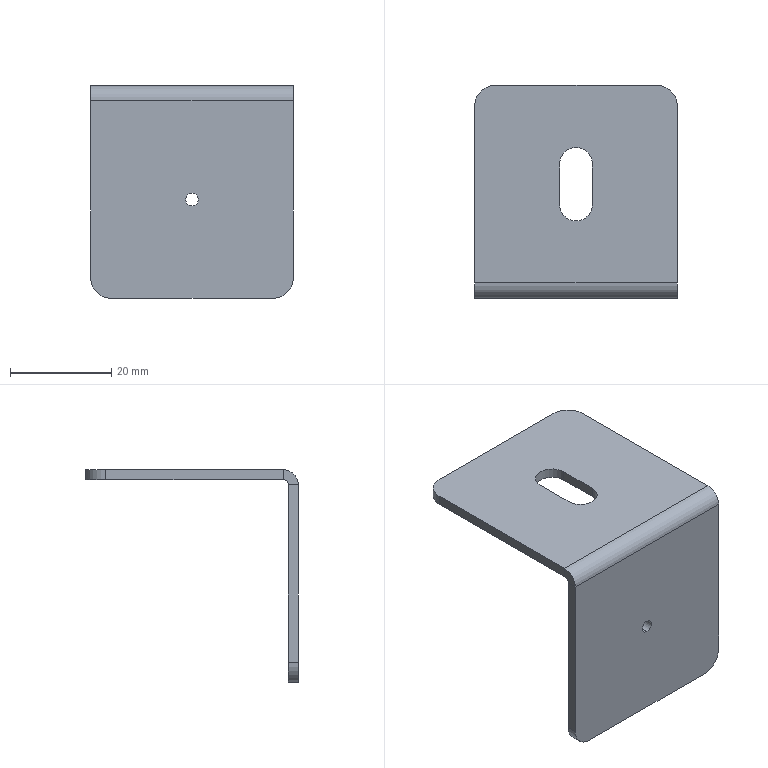Part | SolidWorks | features EdgeFlange 1, Fillet 1, FlatPattern 1, HoleWzd 1, ICE 1, SMBaseFlange 1, SheetMetal 1 | 1 solid | 24 faces | box 40 x 42 x 42 mm | volume 6284 mm3 | plane 14 | cylinder 10 | commonest cylinder face diameters 8 x4 2.5 x2 6.5 x2 2 x1 6 x1
STEP:
#1=CARTESIAN_POINT('',(0.,0.,-2.75));
#2=VERTEX_POINT('',#1);
#3=CARTESIAN_POINT('',(0.,0.,-0.25));
#4=VERTEX_POINT('',#3);
#5=CARTESIAN_POINT('',(0.,0.,-1.5));
#6=DIRECTION('',(0.,1.,0.));
#7=DIRECTION('',(0.,0.,1.));
#8=AXIS2_PLACEMENT_3D('',#5,#6,#7);
#9=CIRCLE('',#8,1.25);
#10=EDGE_CURVE('',#2,#4,#9,.T.);
#11=ORIENTED_EDGE('',*,*,#10,.T.);
#12=CARTESIAN_POINT('',(0.,-2.,-0.25));
#13=VERTEX_POINT('',#12);
#14=CARTESIAN_POINT('',(0.,-2.,-0.25));
#15=DIRECTION('',(0.,-1.,0.));
#16=VECTOR('',#15,1000.);
#17=LINE('',#14,#16);
#18=EDGE_CURVE('',#4,#13,#17,.T.);
#19=ORIENTED_EDGE('',*,*,#18,.T.);
#20=CARTESIAN_POINT('',(0.,-2.,-2.75));
#21=VERTEX_POINT('',#20);
#22=CARTESIAN_POINT('',(0.,-2.,-1.5));
#23=DIRECTION('',(0.,-1.,0.));
#24=DIRECTION('',(0.,0.,-1.));
#25=AXIS2_PLACEMENT_3D('',#22,#23,#24);
#26=CIRCLE('',#25,1.25);
#27=EDGE_CURVE('',#13,#21,#26,.T.);
#28=ORIENTED_EDGE('',*,*,#27,.T.);
#29=CARTESIAN_POINT('',(0.,-2.,-2.75));
#30=DIRECTION('',(0.,-1.,0.));
#31=VECTOR('',#30,1000.);
#32=LINE('',#29,#31);
#33=EDGE_CURVE('',#2,#21,#32,.T.);
#34=ORIENTED_EDGE('',*,*,#33,.F.);
#35=EDGE_LOOP('',(#11,#19,#28,#34));
#36=FACE_OUTER_BOUND('',#35,.T.);
#37=CARTESIAN_POINT('',(0.,-2.,-1.5));
#38=DIRECTION('',(0.,-1.,0.));
#39=DIRECTION('',(0.,0.,-1.));
#40=AXIS2_PLACEMENT_3D('',#37,#38,#39);
#41=CYLINDRICAL_SURFACE('',#40,1.25);
#42=ADVANCED_FACE('',(#36),#41,.F.);
#43=CARTESIAN_POINT('',(20.,-2.,18.));
#44=VERTEX_POINT('',#43);
#45=CARTESIAN_POINT('',(20.,-2.,-17.));
#46=VERTEX_POINT('',#45);
#47=CARTESIAN_POINT('',(20.,-2.,-21.));
#48=DIRECTION('',(0.,0.,-1.));
#49=VECTOR('',#48,1000.);
#50=LINE('',#47,#49);
#51=EDGE_CURVE('',#44,#46,#50,.T.);
#52=ORIENTED_EDGE('',*,*,#51,.T.);
#53=CARTESIAN_POINT('',(20.,0.,-17.));
#54=VERTEX_POINT('',#53);
#55=CARTESIAN_POINT('',(20.,-2.,-17.));
#56=DIRECTION('',(0.,1.,0.));
#57=VECTOR('',#56,1000.);
#58=LINE('',#55,#57);
#59=EDGE_CURVE('',#46,#54,#58,.T.);
#60=ORIENTED_EDGE('',*,*,#59,.T.);
#61=CARTESIAN_POINT('',(20.,0.,18.));
#62=VERTEX_POINT('',#61);
#63=CARTESIAN_POINT('',(20.,0.,-21.));
#64=DIRECTION('',(0.,0.,-1.));
#65=VECTOR('',#64,1000.);
#66=LINE('',#63,#65);
#67=EDGE_CURVE('',#62,#54,#66,.T.);
#68=ORIENTED_EDGE('',*,*,#67,.F.);
#69=CARTESIAN_POINT('',(20.,0.,18.));
#70=DIRECTION('',(0.,-1.,0.));
#71=VECTOR('',#70,1000.);
#72=LINE('',#69,#71);
#73=EDGE_CURVE('',#62,#44,#72,.T.);
#74=ORIENTED_EDGE('',*,*,#73,.T.);
#75=EDGE_LOOP('',(#52,#60,#68,#74));
#76=FACE_OUTER_BOUND('',#75,.T.);
#77=CARTESIAN_POINT('',(20.,-2.,-21.));
#78=DIRECTION('',(1.,0.,0.));
#79=DIRECTION('',(0.,0.,-1.));
#80=AXIS2_PLACEMENT_3D('',#77,#78,#79);
#81=PLANE('',#80);
#82=ADVANCED_FACE('',(#76),#81,.T.);
#83=CARTESIAN_POINT('',(0.,-2.,-1.5));
#84=DIRECTION('',(0.,-1.,0.));
#85=DIRECTION('',(0.,0.,-1.));
#86=AXIS2_PLACEMENT_3D('',#83,#84,#85);
#87=CIRCLE('',#86,1.25);
#88=EDGE_CURVE('',#21,#13,#87,.T.);
#89=ORIENTED_EDGE('',*,*,#88,.F.);
#90=ORIENTED_EDGE('',*,*,#27,.F.);
#91=EDGE_LOOP('',(#89,#90));
#92=FACE_BOUND('',#91,.T.);
#93=CARTESIAN_POINT('',(-20.,-2.,-17.));
#94=VERTEX_POINT('',#93);
#95=CARTESIAN_POINT('',(-20.,-2.,18.));
#96=VERTEX_POINT('',#95);
#97=CARTESIAN_POINT('',(-20.,-2.,-21.));
#98=DIRECTION('',(0.,0.,1.));
#99=VECTOR('',#98,1000.);
#100=LINE('',#97,#99);
#101=EDGE_CURVE('',#94,#96,#100,.T.);
#102=ORIENTED_EDGE('',*,*,#101,.F.);
#103=CARTESIAN_POINT('',(-16.,-2.,-21.));
#104=VERTEX_POINT('',#103);
#105=CARTESIAN_POINT('',(-16.,-2.,-17.));
#106=DIRECTION('',(0.,-1.,0.));
#107=DIRECTION('',(0.,0.,1.));
#108=AXIS2_PLACEMENT_3D('',#105,#106,#107);
#109=CIRCLE('',#108,4.);
#110=EDGE_CURVE('',#94,#104,#109,.T.);
#111=ORIENTED_EDGE('',*,*,#110,.T.);
#112=CARTESIAN_POINT('',(16.,-2.,-21.));
#113=VERTEX_POINT('',#112);
#114=CARTESIAN_POINT('',(-20.,-2.,-21.));
#115=DIRECTION('',(-1.,0.,0.));
#116=VECTOR('',#115,1000.);
#117=LINE('',#114,#116);
#118=EDGE_CURVE('',#113,#104,#117,.T.);
#119=ORIENTED_EDGE('',*,*,#118,.F.);
#120=CARTESIAN_POINT('',(16.,-2.,-17.));
#121=DIRECTION('',(0.,-1.,0.));
#122=DIRECTION('',(0.,0.,1.));
#123=AXIS2_PLACEMENT_3D('',#120,#121,#122);
#124=CIRCLE('',#123,4.);
#125=EDGE_CURVE('',#113,#46,#124,.T.);
#126=ORIENTED_EDGE('',*,*,#125,.T.);
#127=ORIENTED_EDGE('',*,*,#51,.F.);
#128=CARTESIAN_POINT('',(20.,-2.,18.));
#129=DIRECTION('',(-1.,0.,0.));
#130=VECTOR('',#129,1000.);
#131=LINE('',#128,#130);
#132=EDGE_CURVE('',#44,#96,#131,.T.);
#133=ORIENTED_EDGE('',*,*,#132,.T.);
#134=EDGE_LOOP('',(#102,#111,#119,#126,#127,#133));
#135=FACE_OUTER_BOUND('',#134,.T.);
#136=CARTESIAN_POINT('',(0.,-2.,0.));
#137=DIRECTION('',(0.,1.,0.));
#138=DIRECTION('',(0.,0.,1.));
#139=AXIS2_PLACEMENT_3D('',#136,#137,#138);
#140=PLANE('',#139);
#141=ADVANCED_FACE('',(#92,#135),#140,.F.);
#142=ORIENTED_EDGE('',*,*,#10,.F.);
#143=CARTESIAN_POINT('',(0.,0.,-1.5));
#144=DIRECTION('',(0.,1.,0.));
#145=DIRECTION('',(0.,0.,1.));
#146=AXIS2_PLACEMENT_3D('',#143,#144,#145);
#147=CIRCLE('',#146,1.25);
#148=EDGE_CURVE('',#4,#2,#147,.T.);
#149=ORIENTED_EDGE('',*,*,#148,.F.);
#150=EDGE_LOOP('',(#142,#149));
#151=FACE_BOUND('',#150,.T.);
#152=CARTESIAN_POINT('',(16.,0.,-21.));
#153=VERTEX_POINT('',#152);
#154=CARTESIAN_POINT('',(-16.,0.,-21.));
#155=VERTEX_POINT('',#154);
#156=CARTESIAN_POINT('',(-20.,0.,-21.));
#157=DIRECTION('',(-1.,0.,0.));
#158=VECTOR('',#157,1000.);
#159=LINE('',#156,#158);
#160=EDGE_CURVE('',#153,#155,#159,.T.);
#161=ORIENTED_EDGE('',*,*,#160,.T.);
#162=CARTESIAN_POINT('',(-20.,0.,-17.));
#163=VERTEX_POINT('',#162);
#164=CARTESIAN_POINT('',(-16.,0.,-17.));
#165=DIRECTION('',(0.,1.,0.));
#166=DIRECTION('',(0.,0.,1.));
#167=AXIS2_PLACEMENT_3D('',#164,#165,#166);
#168=CIRCLE('',#167,4.);
#169=EDGE_CURVE('',#155,#163,#168,.T.);
#170=ORIENTED_EDGE('',*,*,#169,.T.);
#171=CARTESIAN_POINT('',(-20.,0.,18.));
#172=VERTEX_POINT('',#171);
#173=CARTESIAN_POINT('',(-20.,0.,-21.));
#174=DIRECTION('',(0.,0.,1.));
#175=VECTOR('',#174,1000.);
#176=LINE('',#173,#175);
#177=EDGE_CURVE('',#163,#172,#176,.T.);
#178=ORIENTED_EDGE('',*,*,#177,.T.);
#179=CARTESIAN_POINT('',(20.,0.,18.));
#180=DIRECTION('',(-1.,0.,0.));
#181=VECTOR('',#180,1000.);
#182=LINE('',#179,#181);
#183=EDGE_CURVE('',#62,#172,#182,.T.);
#184=ORIENTED_EDGE('',*,*,#183,.F.);
#185=ORIENTED_EDGE('',*,*,#67,.T.);
#186=CARTESIAN_POINT('',(16.,0.,-17.));
#187=DIRECTION('',(0.,1.,0.));
#188=DIRECTION('',(0.,0.,1.));
#189=AXIS2_PLACEMENT_3D('',#186,#187,#188);
#190=CIRCLE('',#189,4.);
#191=EDGE_CURVE('',#54,#153,#190,.T.);
#192=ORIENTED_EDGE('',*,*,#191,.T.);
#193=EDGE_LOOP('',(#161,#170,#178,#184,#185,#192));
#194=FACE_OUTER_BOUND('',#193,.T.);
#195=CARTESIAN_POINT('',(0.,0.,0.));
#196=DIRECTION('',(0.,1.,0.));
#197=DIRECTION('',(0.,0.,1.));
#198=AXIS2_PLACEMENT_3D('',#195,#196,#197);
#199=PLANE('',#198);
#200=ADVANCED_FACE('',(#151,#194),#199,.T.);
#201=ORIENTED_EDGE('',*,*,#177,.F.);
#202=CARTESIAN_POINT('',(-20.,-2.,-17.));
#203=DIRECTION('',(0.,-1.,0.));
#204=VECTOR('',#203,1000.);
#205=LINE('',#202,#204);
#206=EDGE_CURVE('',#163,#94,#205,.T.);
#207=ORIENTED_EDGE('',*,*,#206,.T.);
#208=ORIENTED_EDGE('',*,*,#101,.T.);
#209=CARTESIAN_POINT('',(-20.,0.,18.));
#210=DIRECTION('',(0.,-1.,0.));
#211=VECTOR('',#210,1000.);
#212=LINE('',#209,#211);
#213=EDGE_CURVE('',#172,#96,#212,.T.);
#214=ORIENTED_EDGE('',*,*,#213,.F.);
#215=EDGE_LOOP('',(#201,#207,#208,#214));
#216=FACE_OUTER_BOUND('',#215,.T.);
#217=CARTESIAN_POINT('',(-20.,-2.,-21.));
#218=DIRECTION('',(-1.,0.,0.));
#219=DIRECTION('',(0.,0.,1.));
#220=AXIS2_PLACEMENT_3D('',#217,#218,#219);
#221=PLANE('',#220);
#222=ADVANCED_FACE('',(#216),#221,.T.);
#223=ORIENTED_EDGE('',*,*,#118,.T.);
#224=CARTESIAN_POINT('',(-16.,-2.,-21.));
#225=DIRECTION('',(0.,1.,0.));
#226=VECTOR('',#225,1000.);
#227=LINE('',#224,#226);
#228=EDGE_CURVE('',#104,#155,#227,.T.);
#229=ORIENTED_EDGE('',*,*,#228,.T.);
#230=ORIENTED_EDGE('',*,*,#160,.F.);
#231=CARTESIAN_POINT('',(16.,-2.,-21.));
#232=DIRECTION('',(0.,-1.,0.));
#233=VECTOR('',#232,1000.);
#234=LINE('',#231,#233);
#235=EDGE_CURVE('',#153,#113,#234,.T.);
#236=ORIENTED_EDGE('',*,*,#235,.T.);
#237=EDGE_LOOP('',(#223,#229,#230,#236));
#238=FACE_OUTER_BOUND('',#237,.T.);
#239=CARTESIAN_POINT('',(-20.,-2.,-21.));
#240=DIRECTION('',(0.,0.,-1.));
#241=DIRECTION('',(-1.,0.,0.));
#242=AXIS2_PLACEMENT_3D('',#239,#240,#241);
#243=PLANE('',#242);
#244=ADVANCED_FACE('',(#238),#243,.T.);
#245=CARTESIAN_POINT('',(-20.,1.,19.));
#246=VERTEX_POINT('',#245);
#247=CARTESIAN_POINT('',(-20.,1.,21.));
#248=VERTEX_POINT('',#247);
#249=CARTESIAN_POINT('',(-20.,1.,21.));
#250=DIRECTION('',(0.,0.,1.));
#251=VECTOR('',#250,1000.);
#252=LINE('',#249,#251);
#253=EDGE_CURVE('',#246,#248,#252,.T.);
#254=ORIENTED_EDGE('',*,*,#253,.F.);
#255=CARTESIAN_POINT('',(-20.,1.,18.));
#256=DIRECTION('',(-1.,0.,0.));
#257=DIRECTION('',(0.,0.,-1.));
#258=AXIS2_PLACEMENT_3D('',#255,#256,#257);
#259=CIRCLE('',#258,1.);
#260=EDGE_CURVE('',#172,#246,#259,.T.);
#261=ORIENTED_EDGE('',*,*,#260,.F.);
#262=ORIENTED_EDGE('',*,*,#213,.T.);
#263=CARTESIAN_POINT('',(-20.,1.,18.));
#264=DIRECTION('',(-1.,0.,0.));
#265=DIRECTION('',(0.,0.,-1.));
#266=AXIS2_PLACEMENT_3D('',#263,#264,#265);
#267=CIRCLE('',#266,3.);
#268=EDGE_CURVE('',#96,#248,#267,.T.);
#269=ORIENTED_EDGE('',*,*,#268,.T.);
#270=EDGE_LOOP('',(#254,#261,#262,#269));
#271=FACE_OUTER_BOUND('',#270,.T.);
#272=CARTESIAN_POINT('',(-20.,1.,18.));
#273=DIRECTION('',(-1.,0.,0.));
#274=DIRECTION('',(0.,0.,1.));
#275=AXIS2_PLACEMENT_3D('',#272,#273,#274);
#276=PLANE('',#275);
#277=ADVANCED_FACE('',(#271),#276,.T.);
#278=CARTESIAN_POINT('',(20.,1.,19.));
#279=VERTEX_POINT('',#278);
#280=CARTESIAN_POINT('',(20.,1.,18.));
#281=DIRECTION('',(1.,0.,0.));
#282=DIRECTION('',(0.,0.,-1.));
#283=AXIS2_PLACEMENT_3D('',#280,#281,#282);
#284=CIRCLE('',#283,1.);
#285=EDGE_CURVE('',#279,#62,#284,.T.);
#286=ORIENTED_EDGE('',*,*,#285,.F.);
#287=CARTESIAN_POINT('',(20.,1.,21.));
#288=VERTEX_POINT('',#287);
#289=CARTESIAN_POINT('',(20.,1.,19.));
#290=DIRECTION('',(0.,0.,1.));
#291=VECTOR('',#290,1000.);
#292=LINE('',#289,#291);
#293=EDGE_CURVE('',#279,#288,#292,.T.);
#294=ORIENTED_EDGE('',*,*,#293,.T.);
#295=CARTESIAN_POINT('',(20.,1.,18.));
#296=DIRECTION('',(1.,0.,0.));
#297=DIRECTION('',(0.,0.,-1.));
#298=AXIS2_PLACEMENT_3D('',#295,#296,#297);
#299=CIRCLE('',#298,3.);
#300=EDGE_CURVE('',#288,#44,#299,.T.);
#301=ORIENTED_EDGE('',*,*,#300,.T.);
#302=ORIENTED_EDGE('',*,*,#73,.F.);
#303=EDGE_LOOP('',(#286,#294,#301,#302));
#304=FACE_OUTER_BOUND('',#303,.T.);
#305=CARTESIAN_POINT('',(20.,1.,18.));
#306=DIRECTION('',(-1.,0.,0.));
#307=DIRECTION('',(0.,0.,1.));
#308=AXIS2_PLACEMENT_3D('',#305,#306,#307);
#309=PLANE('',#308);
#310=ADVANCED_FACE('',(#304),#309,.F.);
#311=ORIENTED_EDGE('',*,*,#132,.F.);
#312=ORIENTED_EDGE('',*,*,#300,.F.);
#313=CARTESIAN_POINT('',(-20.,1.,21.));
#314=DIRECTION('',(-1.,0.,0.));
#315=VECTOR('',#314,1000.);
#316=LINE('',#313,#315);
#317=EDGE_CURVE('',#288,#248,#316,.T.);
#318=ORIENTED_EDGE('',*,*,#317,.T.);
#319=ORIENTED_EDGE('',*,*,#268,.F.);
#320=EDGE_LOOP('',(#311,#312,#318,#319));
#321=FACE_OUTER_BOUND('',#320,.T.);
#322=CARTESIAN_POINT('',(20.,1.,18.));
#323=DIRECTION('',(1.,0.,0.));
#324=DIRECTION('',(0.,0.,1.));
#325=AXIS2_PLACEMENT_3D('',#322,#323,#324);
#326=CYLINDRICAL_SURFACE('',#325,3.);
#327=ADVANCED_FACE('',(#321),#326,.T.);
#328=ORIENTED_EDGE('',*,*,#183,.T.);
#329=ORIENTED_EDGE('',*,*,#260,.T.);
#330=CARTESIAN_POINT('',(-20.,1.,19.));
#331=DIRECTION('',(1.,0.,0.));
#332=VECTOR('',#331,1000.);
#333=LINE('',#330,#332);
#334=EDGE_CURVE('',#246,#279,#333,.T.);
#335=ORIENTED_EDGE('',*,*,#334,.T.);
#336=ORIENTED_EDGE('',*,*,#285,.T.);
#337=EDGE_LOOP('',(#328,#329,#335,#336));
#338=FACE_OUTER_BOUND('',#337,.T.);
#339=CARTESIAN_POINT('',(20.,1.,18.));
#340=DIRECTION('',(1.,0.,0.));
#341=DIRECTION('',(0.,0.,1.));
#342=AXIS2_PLACEMENT_3D('',#339,#340,#341);
#343=CYLINDRICAL_SURFACE('',#342,1.);
#344=ADVANCED_FACE('',(#338),#343,.F.);
#345=CARTESIAN_POINT('',(-20.,36.,21.));
#346=VERTEX_POINT('',#345);
#347=CARTESIAN_POINT('',(-20.,0.,21.));
#348=DIRECTION('',(0.,-1.,0.));
#349=VECTOR('',#348,1000.);
#350=LINE('',#347,#349);
#351=EDGE_CURVE('',#346,#248,#350,.T.);
#352=ORIENTED_EDGE('',*,*,#351,.F.);
#353=CARTESIAN_POINT('',(-20.,36.,19.));
#354=VERTEX_POINT('',#353);
#355=CARTESIAN_POINT('',(-20.,36.,21.));
#356=DIRECTION('',(0.,0.,-1.));
#357=VECTOR('',#356,1000.);
#358=LINE('',#355,#357);
#359=EDGE_CURVE('',#346,#354,#358,.T.);
#360=ORIENTED_EDGE('',*,*,#359,.T.);
#361=CARTESIAN_POINT('',(-20.,0.,19.));
#362=DIRECTION('',(0.,-1.,0.));
#363=VECTOR('',#362,1000.);
#364=LINE('',#361,#363);
#365=EDGE_CURVE('',#354,#246,#364,.T.);
#366=ORIENTED_EDGE('',*,*,#365,.T.);
#367=ORIENTED_EDGE('',*,*,#253,.T.);
#368=EDGE_LOOP('',(#352,#360,#366,#367));
#369=FACE_OUTER_BOUND('',#368,.T.);
#370=CARTESIAN_POINT('',(-20.,0.,21.));
#371=DIRECTION('',(1.,0.,0.));
#372=DIRECTION('',(0.,1.,0.));
#373=AXIS2_PLACEMENT_3D('',#370,#371,#372);
#374=PLANE('',#373);
#375=ADVANCED_FACE('',(#369),#374,.F.);
#376=CARTESIAN_POINT('',(20.,36.,19.));
#377=VERTEX_POINT('',#376);
#378=CARTESIAN_POINT('',(20.,40.,19.));
#379=DIRECTION('',(0.,1.,0.));
#380=VECTOR('',#379,1000.);
#381=LINE('',#378,#380);
#382=EDGE_CURVE('',#279,#377,#381,.T.);
#383=ORIENTED_EDGE('',*,*,#382,.T.);
#384=CARTESIAN_POINT('',(20.,36.,21.));
#385=VERTEX_POINT('',#384);
#386=CARTESIAN_POINT('',(20.,36.,21.));
#387=DIRECTION('',(0.,0.,1.));
#388=VECTOR('',#387,1000.);
#389=LINE('',#386,#388);
#390=EDGE_CURVE('',#377,#385,#389,.T.);
#391=ORIENTED_EDGE('',*,*,#390,.T.);
#392=CARTESIAN_POINT('',(20.,0.,21.));
#393=DIRECTION('',(0.,1.,0.));
#394=VECTOR('',#393,1000.);
#395=LINE('',#392,#394);
#396=EDGE_CURVE('',#288,#385,#395,.T.);
#397=ORIENTED_EDGE('',*,*,#396,.F.);
#398=ORIENTED_EDGE('',*,*,#293,.F.);
#399=EDGE_LOOP('',(#383,#391,#397,#398));
#400=FACE_OUTER_BOUND('',#399,.T.);
#401=CARTESIAN_POINT('',(20.,40.,21.));
#402=DIRECTION('',(-1.,0.,0.));
#403=DIRECTION('',(0.,-1.,0.));
#404=AXIS2_PLACEMENT_3D('',#401,#402,#403);
#405=PLANE('',#404);
#406=ADVANCED_FACE('',(#400),#405,.F.);
#407=CARTESIAN_POINT('',(-3.25,16.5,21.));
#408=VERTEX_POINT('',#407);
#409=CARTESIAN_POINT('',(-3.25,24.5,21.));
#410=VERTEX_POINT('',#409);
#411=CARTESIAN_POINT('',(-3.25,0.,21.));
#412=DIRECTION('',(0.,1.,0.));
#413=VECTOR('',#412,1000.);
#414=LINE('',#411,#413);
#415=EDGE_CURVE('',#408,#410,#414,.T.);
#416=ORIENTED_EDGE('',*,*,#415,.T.);
#417=CARTESIAN_POINT('',(3.25,24.5,21.));
#418=VERTEX_POINT('',#417);
#419=CARTESIAN_POINT('',(0.,24.5,21.));
#420=DIRECTION('',(0.,0.,-1.));
#421=DIRECTION('',(-1.,0.,0.));
#422=AXIS2_PLACEMENT_3D('',#419,#420,#421);
#423=CIRCLE('',#422,3.25);
#424=EDGE_CURVE('',#410,#418,#423,.T.);
#425=ORIENTED_EDGE('',*,*,#424,.T.);
#426=CARTESIAN_POINT('',(3.25,16.5,21.));
#427=VERTEX_POINT('',#426);
#428=CARTESIAN_POINT('',(3.25,0.,21.));
#429=DIRECTION('',(0.,-1.,0.));
#430=VECTOR('',#429,1000.);
#431=LINE('',#428,#430);
#432=EDGE_CURVE('',#418,#427,#431,.T.);
#433=ORIENTED_EDGE('',*,*,#432,.T.);
#434=CARTESIAN_POINT('',(0.,16.5,21.));
#435=DIRECTION('',(0.,0.,-1.));
#436=DIRECTION('',(-1.,0.,0.));
#437=AXIS2_PLACEMENT_3D('',#434,#435,#436);
#438=CIRCLE('',#437,3.25);
#439=EDGE_CURVE('',#427,#408,#438,.T.);
#440=ORIENTED_EDGE('',*,*,#439,.T.);
#441=EDGE_LOOP('',(#416,#425,#433,#440));
#442=FACE_BOUND('',#441,.T.);
#443=CARTESIAN_POINT('',(16.,40.,21.));
#444=VERTEX_POINT('',#443);
#445=CARTESIAN_POINT('',(-16.,40.,21.));
#446=VERTEX_POINT('',#445);
#447=CARTESIAN_POINT('',(0.,40.,21.));
#448=DIRECTION('',(-1.,0.,0.));
#449=VECTOR('',#448,1000.);
#450=LINE('',#447,#449);
#451=EDGE_CURVE('',#444,#446,#450,.T.);
#452=ORIENTED_EDGE('',*,*,#451,.T.);
#453=CARTESIAN_POINT('',(-16.,36.,21.));
#454=DIRECTION('',(0.,0.,1.));
#455=DIRECTION('',(-1.,0.,0.));
#456=AXIS2_PLACEMENT_3D('',#453,#454,#455);
#457=CIRCLE('',#456,4.);
#458=EDGE_CURVE('',#446,#346,#457,.T.);
#459=ORIENTED_EDGE('',*,*,#458,.T.);
#460=ORIENTED_EDGE('',*,*,#351,.T.);
#461=ORIENTED_EDGE('',*,*,#317,.F.);
#462=ORIENTED_EDGE('',*,*,#396,.T.);
#463=CARTESIAN_POINT('',(16.,36.,21.));
#464=DIRECTION('',(0.,0.,1.));
#465=DIRECTION('',(-1.,0.,0.));
#466=AXIS2_PLACEMENT_3D('',#463,#464,#465);
#467=CIRCLE('',#466,4.);
#468=EDGE_CURVE('',#385,#444,#467,.T.);
#469=ORIENTED_EDGE('',*,*,#468,.T.);
#470=EDGE_LOOP('',(#452,#459,#460,#461,#462,#469));
#471=FACE_OUTER_BOUND('',#470,.T.);
#472=CARTESIAN_POINT('',(0.,0.,21.));
#473=DIRECTION('',(0.,0.,-1.));
#474=DIRECTION('',(-1.,0.,0.));
#475=AXIS2_PLACEMENT_3D('',#472,#473,#474);
#476=PLANE('',#475);
#477=ADVANCED_FACE('',(#442,#471),#476,.F.);
#478=CARTESIAN_POINT('',(-3.25,24.5,19.));
#479=VERTEX_POINT('',#478);
#480=CARTESIAN_POINT('',(3.25,24.5,19.));
#481=VERTEX_POINT('',#480);
#482=CARTESIAN_POINT('',(0.,24.5,19.));
#483=DIRECTION('',(0.,0.,-1.));
#484=DIRECTION('',(-1.,0.,0.));
#485=AXIS2_PLACEMENT_3D('',#482,#483,#484);
#486=CIRCLE('',#485,3.25);
#487=EDGE_CURVE('',#479,#481,#486,.T.);
#488=ORIENTED_EDGE('',*,*,#487,.F.);
#489=CARTESIAN_POINT('',(-3.25,16.5,19.));
#490=VERTEX_POINT('',#489);
#491=CARTESIAN_POINT('',(-3.25,24.5,19.));
#492=DIRECTION('',(0.,1.,0.));
#493=VECTOR('',#492,1000.);
#494=LINE('',#491,#493);
#495=EDGE_CURVE('',#490,#479,#494,.T.);
#496=ORIENTED_EDGE('',*,*,#495,.F.);
#497=CARTESIAN_POINT('',(3.25,16.5,19.));
#498=VERTEX_POINT('',#497);
#499=CARTESIAN_POINT('',(0.,16.5,19.));
#500=DIRECTION('',(0.,0.,-1.));
#501=DIRECTION('',(-1.,0.,0.));
#502=AXIS2_PLACEMENT_3D('',#499,#500,#501);
#503=CIRCLE('',#502,3.25);
#504=EDGE_CURVE('',#498,#490,#503,.T.);
#505=ORIENTED_EDGE('',*,*,#504,.F.);
#506=CARTESIAN_POINT('',(3.25,24.5,19.));
#507=DIRECTION('',(0.,-1.,0.));
#508=VECTOR('',#507,1000.);
#509=LINE('',#506,#508);
#510=EDGE_CURVE('',#481,#498,#509,.T.);
#511=ORIENTED_EDGE('',*,*,#510,.F.);
#512=EDGE_LOOP('',(#488,#496,#505,#511));
#513=FACE_BOUND('',#512,.T.);
#514=ORIENTED_EDGE('',*,*,#365,.F.);
#515=CARTESIAN_POINT('',(-16.,40.,19.));
#516=VERTEX_POINT('',#515);
#517=CARTESIAN_POINT('',(-16.,36.,19.));
#518=DIRECTION('',(0.,0.,-1.));
#519=DIRECTION('',(-1.,0.,0.));
#520=AXIS2_PLACEMENT_3D('',#517,#518,#519);
#521=CIRCLE('',#520,4.);
#522=EDGE_CURVE('',#354,#516,#521,.T.);
#523=ORIENTED_EDGE('',*,*,#522,.T.);
#524=CARTESIAN_POINT('',(16.,40.,19.));
#525=VERTEX_POINT('',#524);
#526=CARTESIAN_POINT('',(-20.,40.,19.));
#527=DIRECTION('',(-1.,0.,0.));
#528=VECTOR('',#527,1000.);
#529=LINE('',#526,#528);
#530=EDGE_CURVE('',#525,#516,#529,.T.);
#531=ORIENTED_EDGE('',*,*,#530,.F.);
#532=CARTESIAN_POINT('',(16.,36.,19.));
#533=DIRECTION('',(0.,0.,-1.));
#534=DIRECTION('',(-1.,0.,0.));
#535=AXIS2_PLACEMENT_3D('',#532,#533,#534);
#536=CIRCLE('',#535,4.);
#537=EDGE_CURVE('',#525,#377,#536,.T.);
#538=ORIENTED_EDGE('',*,*,#537,.T.);
#539=ORIENTED_EDGE('',*,*,#382,.F.);
#540=ORIENTED_EDGE('',*,*,#334,.F.);
#541=EDGE_LOOP('',(#514,#523,#531,#538,#539,#540));
#542=FACE_OUTER_BOUND('',#541,.T.);
#543=CARTESIAN_POINT('',(0.,0.,19.));
#544=DIRECTION('',(0.,0.,-1.));
#545=DIRECTION('',(-1.,0.,0.));
#546=AXIS2_PLACEMENT_3D('',#543,#544,#545);
#547=PLANE('',#546);
#548=ADVANCED_FACE('',(#513,#542),#547,.T.);
#549=ORIENTED_EDGE('',*,*,#530,.T.);
#550=CARTESIAN_POINT('',(-16.,40.,21.));
#551=DIRECTION('',(0.,0.,1.));
#552=VECTOR('',#551,1000.);
#553=LINE('',#550,#552);
#554=EDGE_CURVE('',#516,#446,#553,.T.);
#555=ORIENTED_EDGE('',*,*,#554,.T.);
#556=ORIENTED_EDGE('',*,*,#451,.F.);
#557=CARTESIAN_POINT('',(16.,40.,21.));
#558=DIRECTION('',(0.,0.,-1.));
#559=VECTOR('',#558,1000.);
#560=LINE('',#557,#559);
#561=EDGE_CURVE('',#444,#525,#560,.T.);
#562=ORIENTED_EDGE('',*,*,#561,.T.);
#563=EDGE_LOOP('',(#549,#555,#556,#562));
#564=FACE_OUTER_BOUND('',#563,.T.);
#565=CARTESIAN_POINT('',(-20.,40.,21.));
#566=DIRECTION('',(0.,-1.,0.));
#567=DIRECTION('',(0.,0.,-1.));
#568=AXIS2_PLACEMENT_3D('',#565,#566,#567);
#569=PLANE('',#568);
#570=ADVANCED_FACE('',(#564),#569,.F.);
#571=CARTESIAN_POINT('',(-3.25,24.5,29.));
#572=DIRECTION('',(0.,0.,-1.));
#573=VECTOR('',#572,1000.);
#574=LINE('',#571,#573);
#575=EDGE_CURVE('',#410,#479,#574,.T.);
#576=ORIENTED_EDGE('',*,*,#575,.T.);
#577=ORIENTED_EDGE('',*,*,#487,.T.);
#578=CARTESIAN_POINT('',(3.25,24.5,29.));
#579=DIRECTION('',(0.,0.,-1.));
#580=VECTOR('',#579,1000.);
#581=LINE('',#578,#580);
#582=EDGE_CURVE('',#418,#481,#581,.T.);
#583=ORIENTED_EDGE('',*,*,#582,.F.);
#584=ORIENTED_EDGE('',*,*,#424,.F.);
#585=EDGE_LOOP('',(#576,#577,#583,#584));
#586=FACE_OUTER_BOUND('',#585,.T.);
#587=CARTESIAN_POINT('',(0.,24.5,29.));
#588=DIRECTION('',(0.,0.,-1.));
#589=DIRECTION('',(-1.,0.,0.));
#590=AXIS2_PLACEMENT_3D('',#587,#588,#589);
#591=CYLINDRICAL_SURFACE('',#590,3.25);
#592=ADVANCED_FACE('',(#586),#591,.F.);
#593=CARTESIAN_POINT('',(-3.25,16.5,29.));
#594=DIRECTION('',(0.,0.,-1.));
#595=VECTOR('',#594,1000.);
#596=LINE('',#593,#595);
#597=EDGE_CURVE('',#408,#490,#596,.T.);
#598=ORIENTED_EDGE('',*,*,#597,.T.);
#599=ORIENTED_EDGE('',*,*,#495,.T.);
#600=ORIENTED_EDGE('',*,*,#575,.F.);
#601=ORIENTED_EDGE('',*,*,#415,.F.);
#602=EDGE_LOOP('',(#598,#599,#600,#601));
#603=FACE_OUTER_BOUND('',#602,.T.);
#604=CARTESIAN_POINT('',(-3.25,24.5,29.));
#605=DIRECTION('',(-1.,0.,0.));
#606=DIRECTION('',(0.,0.,1.));
#607=AXIS2_PLACEMENT_3D('',#604,#605,#606);
#608=PLANE('',#607);
#609=ADVANCED_FACE('',(#603),#608,.F.);
#610=CARTESIAN_POINT('',(3.25,16.5,29.));
#611=DIRECTION('',(0.,0.,-1.));
#612=VECTOR('',#611,1000.);
#613=LINE('',#610,#612);
#614=EDGE_CURVE('',#427,#498,#613,.T.);
#615=ORIENTED_EDGE('',*,*,#614,.T.);
#616=ORIENTED_EDGE('',*,*,#504,.T.);
#617=ORIENTED_EDGE('',*,*,#597,.F.);
#618=ORIENTED_EDGE('',*,*,#439,.F.);
#619=EDGE_LOOP('',(#615,#616,#617,#618));
#620=FACE_OUTER_BOUND('',#619,.T.);
#621=CARTESIAN_POINT('',(0.,16.5,29.));
#622=DIRECTION('',(0.,0.,-1.));
#623=DIRECTION('',(-1.,0.,0.));
#624=AXIS2_PLACEMENT_3D('',#621,#622,#623);
#625=CYLINDRICAL_SURFACE('',#624,3.25);
#626=ADVANCED_FACE('',(#620),#625,.F.);
#627=ORIENTED_EDGE('',*,*,#582,.T.);
#628=ORIENTED_EDGE('',*,*,#510,.T.);
#629=ORIENTED_EDGE('',*,*,#614,.F.);
#630=ORIENTED_EDGE('',*,*,#432,.F.);
#631=EDGE_LOOP('',(#627,#628,#629,#630));
#632=FACE_OUTER_BOUND('',#631,.T.);
#633=CARTESIAN_POINT('',(3.25,24.5,29.));
#634=DIRECTION('',(1.,0.,0.));
#635=DIRECTION('',(0.,0.,-1.));
#636=AXIS2_PLACEMENT_3D('',#633,#634,#635);
#637=PLANE('',#636);
#638=ADVANCED_FACE('',(#632),#637,.F.);
#639=ORIENTED_EDGE('',*,*,#18,.F.);
#640=ORIENTED_EDGE('',*,*,#148,.T.);
#641=ORIENTED_EDGE('',*,*,#33,.T.);
#642=ORIENTED_EDGE('',*,*,#88,.T.);
#643=EDGE_LOOP('',(#639,#640,#641,#642));
#644=FACE_OUTER_BOUND('',#643,.T.);
#645=CARTESIAN_POINT('',(0.,-2.,-1.5));
#646=DIRECTION('',(0.,-1.,0.));
#647=DIRECTION('',(0.,0.,-1.));
#648=AXIS2_PLACEMENT_3D('',#645,#646,#647);
#649=CYLINDRICAL_SURFACE('',#648,1.25);
#650=ADVANCED_FACE('',(#644),#649,.F.);
#651=ORIENTED_EDGE('',*,*,#110,.F.);
#652=ORIENTED_EDGE('',*,*,#206,.F.);
#653=ORIENTED_EDGE('',*,*,#169,.F.);
#654=ORIENTED_EDGE('',*,*,#228,.F.);
#655=EDGE_LOOP('',(#651,#652,#653,#654));
#656=FACE_OUTER_BOUND('',#655,.T.);
#657=CARTESIAN_POINT('',(-16.,-2.,-17.));
#658=DIRECTION('',(0.,1.,0.));
#659=DIRECTION('',(0.,0.,1.));
#660=AXIS2_PLACEMENT_3D('',#657,#658,#659);
#661=CYLINDRICAL_SURFACE('',#660,4.);
#662=ADVANCED_FACE('',(#656),#661,.T.);
#663=ORIENTED_EDGE('',*,*,#458,.F.);
#664=ORIENTED_EDGE('',*,*,#554,.F.);
#665=ORIENTED_EDGE('',*,*,#522,.F.);
#666=ORIENTED_EDGE('',*,*,#359,.F.);
#667=EDGE_LOOP('',(#663,#664,#665,#666));
#668=FACE_OUTER_BOUND('',#667,.T.);
#669=CARTESIAN_POINT('',(-16.,36.,21.));
#670=DIRECTION('',(0.,0.,-1.));
#671=DIRECTION('',(-1.,0.,0.));
#672=AXIS2_PLACEMENT_3D('',#669,#670,#671);
#673=CYLINDRICAL_SURFACE('',#672,4.);
#674=ADVANCED_FACE('',(#668),#673,.T.);
#675=ORIENTED_EDGE('',*,*,#125,.F.);
#676=ORIENTED_EDGE('',*,*,#235,.F.);
#677=ORIENTED_EDGE('',*,*,#191,.F.);
#678=ORIENTED_EDGE('',*,*,#59,.F.);
#679=EDGE_LOOP('',(#675,#676,#677,#678));
#680=FACE_OUTER_BOUND('',#679,.T.);
#681=CARTESIAN_POINT('',(16.,-2.,-17.));
#682=DIRECTION('',(0.,1.,0.));
#683=DIRECTION('',(0.,0.,1.));
#684=AXIS2_PLACEMENT_3D('',#681,#682,#683);
#685=CYLINDRICAL_SURFACE('',#684,4.);
#686=ADVANCED_FACE('',(#680),#685,.T.);
#687=ORIENTED_EDGE('',*,*,#468,.F.);
#688=ORIENTED_EDGE('',*,*,#390,.F.);
#689=ORIENTED_EDGE('',*,*,#537,.F.);
#690=ORIENTED_EDGE('',*,*,#561,.F.);
#691=EDGE_LOOP('',(#687,#688,#689,#690));
#692=FACE_OUTER_BOUND('',#691,.T.);
#693=CARTESIAN_POINT('',(16.,36.,21.));
#694=DIRECTION('',(0.,0.,-1.));
#695=DIRECTION('',(-1.,0.,0.));
#696=AXIS2_PLACEMENT_3D('',#693,#694,#695);
#697=CYLINDRICAL_SURFACE('',#696,4.);
#698=ADVANCED_FACE('',(#692),#697,.T.);
#699=CLOSED_SHELL('',(#42,#82,#141,#200,#222,#244,#277,#310,#327,#344,#375,#406,#477,#548,#570,#592,#609,#626,#638,#650,#662,#674,#686,#698));
#700=MANIFOLD_SOLID_BREP('',#699);
#701=CARTESIAN_POINT('',(0.,0.,0.));
#702=DIRECTION('',(0.,0.,1.));
#703=DIRECTION('',(1.,0.,0.));
#704=AXIS2_PLACEMENT_3D('',#701,#702,#703);
#705=(LENGTH_UNIT()NAMED_UNIT(*)SI_UNIT(.MILLI.,.METRE.));
#706=UNCERTAINTY_MEASURE_WITH_UNIT(LENGTH_MEASURE(0.00001),#705,'','');
#707=(NAMED_UNIT(*)PLANE_ANGLE_UNIT()SI_UNIT($,.RADIAN.));
#708=(NAMED_UNIT(*)SI_UNIT($,.STERADIAN.)SOLID_ANGLE_UNIT());
#709=(GEOMETRIC_REPRESENTATION_CONTEXT(3)GLOBAL_UNCERTAINTY_ASSIGNED_CONTEXT((#706))GLOBAL_UNIT_ASSIGNED_CONTEXT((#705,#707,#708))REPRESENTATION_CONTEXT('',''));
#710=ADVANCED_BREP_SHAPE_REPRESENTATION('',(#700,#704),#709);